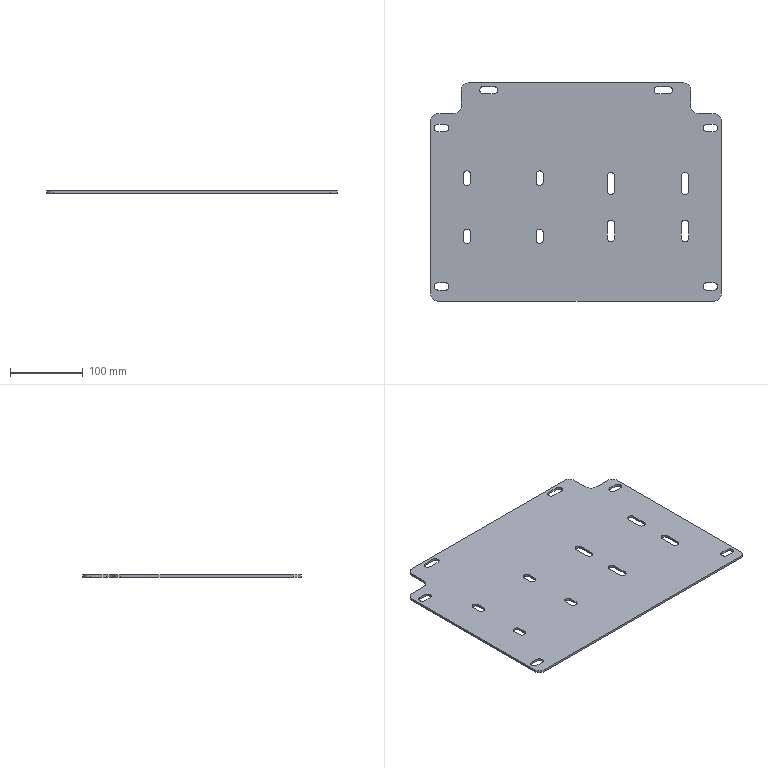Part | SolidWorks | features ICE 3, Extrusion 1, Fillet 1 | 1 solid | 80 faces | box 400 x 300 x 3 mm | volume 340160 mm3 | cylinder 42 | plane 38 | commonest cylinder face diameters 10 x34 20 x8